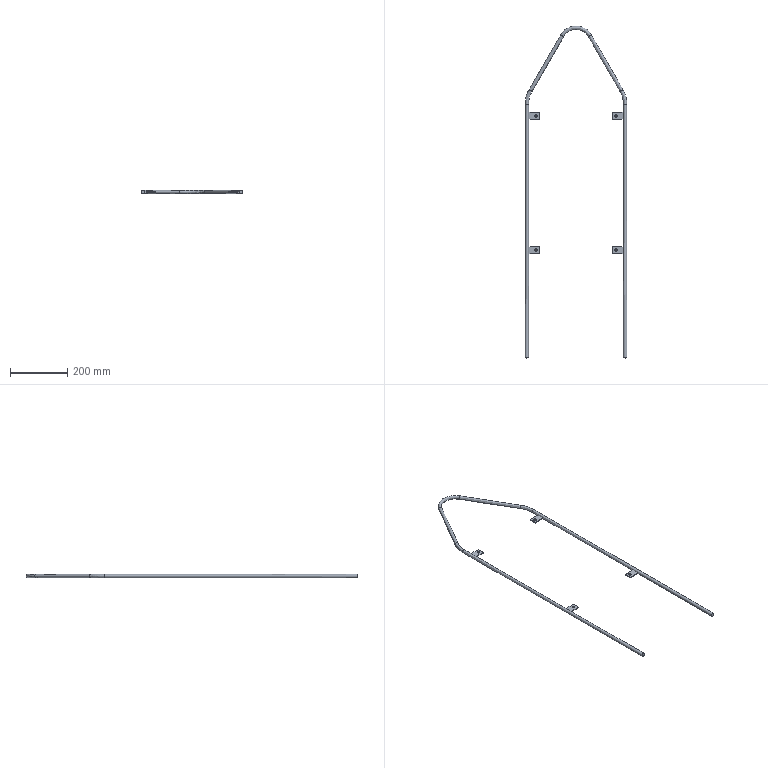Part | NX | features DATUM_CSYS 1, DATUM_PLANE 1, EXTRUDE 1, SKETCH 1, SWP104 1 | 5 solids | 37 faces | box 356.002 x 1162 x 12 mm | volume 288211 mm3 | plane 26 | spline 7 | cylinder 4 | commonest cylinder face diameters 9 x4